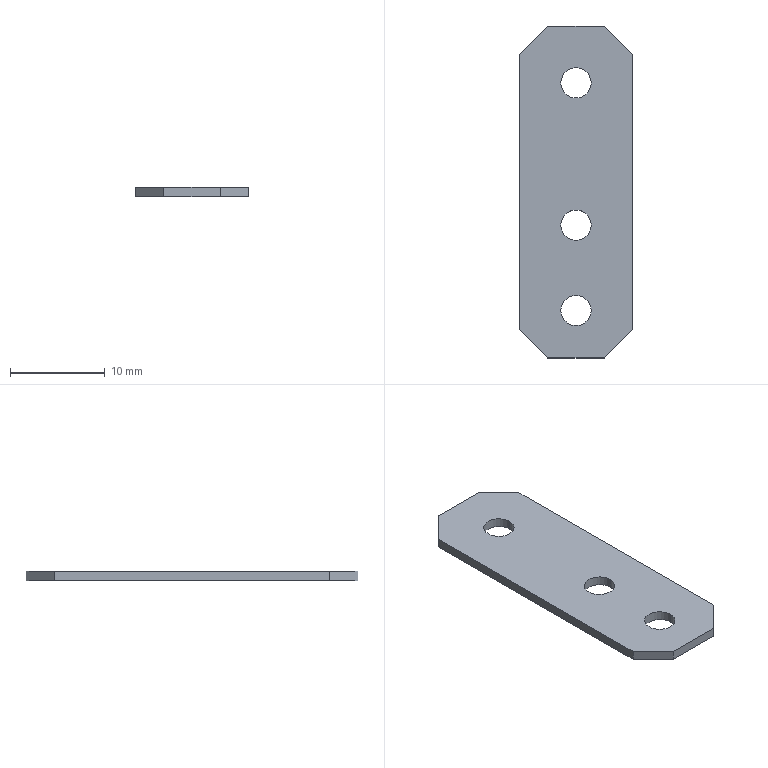Part | SolidWorks | features BaseBody 1 | 1 solid | 16 faces | box 12 x 35 x 1 mm | volume 377.873 mm3 | plane 10 | cylinder 6 | commonest cylinder face diameters 3.2 x6
STEP:
#1=CARTESIAN_POINT('',(1.6,-12.5,-1.));
#2=VERTEX_POINT('',#1);
#3=CARTESIAN_POINT('',(-1.6,-12.5,-1.));
#4=VERTEX_POINT('',#3);
#5=CARTESIAN_POINT('',(0.,-12.5,-1.));
#6=DIRECTION('',(0.,0.,-1.));
#7=DIRECTION('',(1.,0.,0.));
#8=AXIS2_PLACEMENT_3D('',#5,#6,#7);
#9=CIRCLE('',#8,1.6);
#10=EDGE_CURVE('',#2,#4,#9,.T.);
#11=ORIENTED_EDGE('',*,*,#10,.T.);
#12=CARTESIAN_POINT('',(-1.6,-12.5,0.));
#13=VERTEX_POINT('',#12);
#14=CARTESIAN_POINT('',(-1.6,-12.5,-1.));
#15=DIRECTION('',(0.,0.,1.));
#16=VECTOR('',#15,1000.);
#17=LINE('',#14,#16);
#18=EDGE_CURVE('',#4,#13,#17,.T.);
#19=ORIENTED_EDGE('',*,*,#18,.T.);
#20=CARTESIAN_POINT('',(1.6,-12.5,0.));
#21=VERTEX_POINT('',#20);
#22=CARTESIAN_POINT('',(0.,-12.5,0.));
#23=DIRECTION('',(0.,0.,1.));
#24=DIRECTION('',(1.,0.,0.));
#25=AXIS2_PLACEMENT_3D('',#22,#23,#24);
#26=CIRCLE('',#25,1.6);
#27=EDGE_CURVE('',#13,#21,#26,.T.);
#28=ORIENTED_EDGE('',*,*,#27,.T.);
#29=CARTESIAN_POINT('',(1.6,-12.5,-1.));
#30=DIRECTION('',(0.,0.,1.));
#31=VECTOR('',#30,1000.);
#32=LINE('',#29,#31);
#33=EDGE_CURVE('',#2,#21,#32,.T.);
#34=ORIENTED_EDGE('',*,*,#33,.F.);
#35=EDGE_LOOP('',(#11,#19,#28,#34));
#36=FACE_OUTER_BOUND('',#35,.T.);
#37=CARTESIAN_POINT('',(0.,-12.5,-1.));
#38=DIRECTION('',(0.,0.,1.));
#39=DIRECTION('',(1.,0.,0.));
#40=AXIS2_PLACEMENT_3D('',#37,#38,#39);
#41=CYLINDRICAL_SURFACE('',#40,1.6);
#42=ADVANCED_FACE('',(#36),#41,.F.);
#43=CARTESIAN_POINT('',(1.6,11.5,-1.));
#44=VERTEX_POINT('',#43);
#45=CARTESIAN_POINT('',(-1.6,11.5,-1.));
#46=VERTEX_POINT('',#45);
#47=CARTESIAN_POINT('',(0.,11.5,-1.));
#48=DIRECTION('',(0.,0.,-1.));
#49=DIRECTION('',(1.,0.,0.));
#50=AXIS2_PLACEMENT_3D('',#47,#48,#49);
#51=CIRCLE('',#50,1.6);
#52=EDGE_CURVE('',#44,#46,#51,.T.);
#53=ORIENTED_EDGE('',*,*,#52,.T.);
#54=CARTESIAN_POINT('',(-1.6,11.5,0.));
#55=VERTEX_POINT('',#54);
#56=CARTESIAN_POINT('',(-1.6,11.5,-1.));
#57=DIRECTION('',(0.,0.,1.));
#58=VECTOR('',#57,1000.);
#59=LINE('',#56,#58);
#60=EDGE_CURVE('',#46,#55,#59,.T.);
#61=ORIENTED_EDGE('',*,*,#60,.T.);
#62=CARTESIAN_POINT('',(1.6,11.5,0.));
#63=VERTEX_POINT('',#62);
#64=CARTESIAN_POINT('',(0.,11.5,0.));
#65=DIRECTION('',(0.,0.,-1.));
#66=DIRECTION('',(1.,0.,0.));
#67=AXIS2_PLACEMENT_3D('',#64,#65,#66);
#68=CIRCLE('',#67,1.6);
#69=EDGE_CURVE('',#63,#55,#68,.T.);
#70=ORIENTED_EDGE('',*,*,#69,.F.);
#71=CARTESIAN_POINT('',(1.6,11.5,-1.));
#72=DIRECTION('',(0.,0.,1.));
#73=VECTOR('',#72,1000.);
#74=LINE('',#71,#73);
#75=EDGE_CURVE('',#44,#63,#74,.T.);
#76=ORIENTED_EDGE('',*,*,#75,.F.);
#77=EDGE_LOOP('',(#53,#61,#70,#76));
#78=FACE_OUTER_BOUND('',#77,.T.);
#79=CARTESIAN_POINT('',(0.,11.5,-1.));
#80=DIRECTION('',(0.,0.,1.));
#81=DIRECTION('',(1.,0.,0.));
#82=AXIS2_PLACEMENT_3D('',#79,#80,#81);
#83=CYLINDRICAL_SURFACE('',#82,1.6);
#84=ADVANCED_FACE('',(#78),#83,.F.);
#85=CARTESIAN_POINT('',(1.6,-3.5,-1.));
#86=VERTEX_POINT('',#85);
#87=CARTESIAN_POINT('',(-1.6,-3.5,-1.));
#88=VERTEX_POINT('',#87);
#89=CARTESIAN_POINT('',(0.,-3.5,-1.));
#90=DIRECTION('',(0.,0.,-1.));
#91=DIRECTION('',(1.,0.,0.));
#92=AXIS2_PLACEMENT_3D('',#89,#90,#91);
#93=CIRCLE('',#92,1.6);
#94=EDGE_CURVE('',#86,#88,#93,.T.);
#95=ORIENTED_EDGE('',*,*,#94,.T.);
#96=CARTESIAN_POINT('',(-1.6,-3.5,0.));
#97=VERTEX_POINT('',#96);
#98=CARTESIAN_POINT('',(-1.6,-3.5,-1.));
#99=DIRECTION('',(0.,0.,1.));
#100=VECTOR('',#99,1000.);
#101=LINE('',#98,#100);
#102=EDGE_CURVE('',#88,#97,#101,.T.);
#103=ORIENTED_EDGE('',*,*,#102,.T.);
#104=CARTESIAN_POINT('',(1.6,-3.5,0.));
#105=VERTEX_POINT('',#104);
#106=CARTESIAN_POINT('',(0.,-3.5,0.));
#107=DIRECTION('',(0.,0.,-1.));
#108=DIRECTION('',(1.,0.,0.));
#109=AXIS2_PLACEMENT_3D('',#106,#107,#108);
#110=CIRCLE('',#109,1.6);
#111=EDGE_CURVE('',#105,#97,#110,.T.);
#112=ORIENTED_EDGE('',*,*,#111,.F.);
#113=CARTESIAN_POINT('',(1.6,-3.5,-1.));
#114=DIRECTION('',(0.,0.,1.));
#115=VECTOR('',#114,1000.);
#116=LINE('',#113,#115);
#117=EDGE_CURVE('',#86,#105,#116,.T.);
#118=ORIENTED_EDGE('',*,*,#117,.F.);
#119=EDGE_LOOP('',(#95,#103,#112,#118));
#120=FACE_OUTER_BOUND('',#119,.T.);
#121=CARTESIAN_POINT('',(0.,-3.5,-1.));
#122=DIRECTION('',(0.,0.,1.));
#123=DIRECTION('',(1.,0.,0.));
#124=AXIS2_PLACEMENT_3D('',#121,#122,#123);
#125=CYLINDRICAL_SURFACE('',#124,1.6);
#126=ADVANCED_FACE('',(#120),#125,.F.);
#127=ORIENTED_EDGE('',*,*,#18,.F.);
#128=CARTESIAN_POINT('',(0.,-12.5,-1.));
#129=DIRECTION('',(0.,0.,-1.));
#130=DIRECTION('',(1.,0.,0.));
#131=AXIS2_PLACEMENT_3D('',#128,#129,#130);
#132=CIRCLE('',#131,1.6);
#133=EDGE_CURVE('',#4,#2,#132,.T.);
#134=ORIENTED_EDGE('',*,*,#133,.T.);
#135=ORIENTED_EDGE('',*,*,#33,.T.);
#136=CARTESIAN_POINT('',(0.,-12.5,0.));
#137=DIRECTION('',(0.,0.,1.));
#138=DIRECTION('',(1.,0.,0.));
#139=AXIS2_PLACEMENT_3D('',#136,#137,#138);
#140=CIRCLE('',#139,1.6);
#141=EDGE_CURVE('',#21,#13,#140,.T.);
#142=ORIENTED_EDGE('',*,*,#141,.T.);
#143=EDGE_LOOP('',(#127,#134,#135,#142));
#144=FACE_OUTER_BOUND('',#143,.T.);
#145=CARTESIAN_POINT('',(0.,-12.5,-1.));
#146=DIRECTION('',(0.,0.,1.));
#147=DIRECTION('',(1.,0.,0.));
#148=AXIS2_PLACEMENT_3D('',#145,#146,#147);
#149=CYLINDRICAL_SURFACE('',#148,1.6);
#150=ADVANCED_FACE('',(#144),#149,.F.);
#151=ORIENTED_EDGE('',*,*,#69,.T.);
#152=CARTESIAN_POINT('',(0.,11.5,0.));
#153=DIRECTION('',(0.,0.,-1.));
#154=DIRECTION('',(1.,0.,0.));
#155=AXIS2_PLACEMENT_3D('',#152,#153,#154);
#156=CIRCLE('',#155,1.6);
#157=EDGE_CURVE('',#55,#63,#156,.T.);
#158=ORIENTED_EDGE('',*,*,#157,.T.);
#159=EDGE_LOOP('',(#151,#158));
#160=FACE_BOUND('',#159,.T.);
#161=ORIENTED_EDGE('',*,*,#111,.T.);
#162=CARTESIAN_POINT('',(0.,-3.5,0.));
#163=DIRECTION('',(0.,0.,-1.));
#164=DIRECTION('',(1.,0.,0.));
#165=AXIS2_PLACEMENT_3D('',#162,#163,#164);
#166=CIRCLE('',#165,1.6);
#167=EDGE_CURVE('',#97,#105,#166,.T.);
#168=ORIENTED_EDGE('',*,*,#167,.T.);
#169=EDGE_LOOP('',(#161,#168));
#170=FACE_BOUND('',#169,.T.);
#171=ORIENTED_EDGE('',*,*,#141,.F.);
#172=ORIENTED_EDGE('',*,*,#27,.F.);
#173=EDGE_LOOP('',(#171,#172));
#174=FACE_BOUND('',#173,.T.);
#175=CARTESIAN_POINT('',(6.,-14.5,0.));
#176=VERTEX_POINT('',#175);
#177=CARTESIAN_POINT('',(6.,14.5,0.));
#178=VERTEX_POINT('',#177);
#179=CARTESIAN_POINT('',(6.,0.,0.));
#180=DIRECTION('',(0.,1.,0.));
#181=VECTOR('',#180,1000.);
#182=LINE('',#179,#181);
#183=EDGE_CURVE('',#176,#178,#182,.T.);
#184=ORIENTED_EDGE('',*,*,#183,.T.);
#185=CARTESIAN_POINT('',(3.,17.5,0.));
#186=VERTEX_POINT('',#185);
#187=CARTESIAN_POINT('',(6.,14.5,0.));
#188=DIRECTION('',(-0.7071,0.7071,0.));
#189=VECTOR('',#188,1000.);
#190=LINE('',#187,#189);
#191=EDGE_CURVE('',#178,#186,#190,.T.);
#192=ORIENTED_EDGE('',*,*,#191,.T.);
#193=CARTESIAN_POINT('',(-3.,17.5,0.));
#194=VERTEX_POINT('',#193);
#195=CARTESIAN_POINT('',(0.,17.5,0.));
#196=DIRECTION('',(-1.,0.,0.));
#197=VECTOR('',#196,1000.);
#198=LINE('',#195,#197);
#199=EDGE_CURVE('',#186,#194,#198,.T.);
#200=ORIENTED_EDGE('',*,*,#199,.T.);
#201=CARTESIAN_POINT('',(-6.,14.5,0.));
#202=VERTEX_POINT('',#201);
#203=CARTESIAN_POINT('',(-3.,17.5,0.));
#204=DIRECTION('',(-0.7071,-0.7071,0.));
#205=VECTOR('',#204,1000.);
#206=LINE('',#203,#205);
#207=EDGE_CURVE('',#194,#202,#206,.T.);
#208=ORIENTED_EDGE('',*,*,#207,.T.);
#209=CARTESIAN_POINT('',(-6.,-14.5,0.));
#210=VERTEX_POINT('',#209);
#211=CARTESIAN_POINT('',(-6.,0.,0.));
#212=DIRECTION('',(0.,-1.,0.));
#213=VECTOR('',#212,1000.);
#214=LINE('',#211,#213);
#215=EDGE_CURVE('',#202,#210,#214,.T.);
#216=ORIENTED_EDGE('',*,*,#215,.T.);
#217=CARTESIAN_POINT('',(-3.,-17.5,0.));
#218=VERTEX_POINT('',#217);
#219=CARTESIAN_POINT('',(-6.,-14.5,0.));
#220=DIRECTION('',(0.7071,-0.7071,0.));
#221=VECTOR('',#220,1000.);
#222=LINE('',#219,#221);
#223=EDGE_CURVE('',#210,#218,#222,.T.);
#224=ORIENTED_EDGE('',*,*,#223,.T.);
#225=CARTESIAN_POINT('',(3.,-17.5,0.));
#226=VERTEX_POINT('',#225);
#227=CARTESIAN_POINT('',(0.,-17.5,0.));
#228=DIRECTION('',(1.,0.,0.));
#229=VECTOR('',#228,1000.);
#230=LINE('',#227,#229);
#231=EDGE_CURVE('',#218,#226,#230,.T.);
#232=ORIENTED_EDGE('',*,*,#231,.T.);
#233=CARTESIAN_POINT('',(3.,-17.5,0.));
#234=DIRECTION('',(0.7071,0.7071,0.));
#235=VECTOR('',#234,1000.);
#236=LINE('',#233,#235);
#237=EDGE_CURVE('',#226,#176,#236,.T.);
#238=ORIENTED_EDGE('',*,*,#237,.T.);
#239=EDGE_LOOP('',(#184,#192,#200,#208,#216,#224,#232,#238));
#240=FACE_OUTER_BOUND('',#239,.T.);
#241=CARTESIAN_POINT('',(-6.,-17.5,0.));
#242=DIRECTION('',(0.,0.,1.));
#243=DIRECTION('',(1.,0.,0.));
#244=AXIS2_PLACEMENT_3D('',#241,#242,#243);
#245=PLANE('',#244);
#246=ADVANCED_FACE('',(#160,#170,#174,#240),#245,.T.);
#247=ORIENTED_EDGE('',*,*,#52,.F.);
#248=CARTESIAN_POINT('',(0.,11.5,-1.));
#249=DIRECTION('',(0.,0.,-1.));
#250=DIRECTION('',(1.,0.,0.));
#251=AXIS2_PLACEMENT_3D('',#248,#249,#250);
#252=CIRCLE('',#251,1.6);
#253=EDGE_CURVE('',#46,#44,#252,.T.);
#254=ORIENTED_EDGE('',*,*,#253,.F.);
#255=EDGE_LOOP('',(#247,#254));
#256=FACE_BOUND('',#255,.T.);
#257=ORIENTED_EDGE('',*,*,#94,.F.);
#258=CARTESIAN_POINT('',(0.,-3.5,-1.));
#259=DIRECTION('',(0.,0.,-1.));
#260=DIRECTION('',(1.,0.,0.));
#261=AXIS2_PLACEMENT_3D('',#258,#259,#260);
#262=CIRCLE('',#261,1.6);
#263=EDGE_CURVE('',#88,#86,#262,.T.);
#264=ORIENTED_EDGE('',*,*,#263,.F.);
#265=EDGE_LOOP('',(#257,#264));
#266=FACE_BOUND('',#265,.T.);
#267=ORIENTED_EDGE('',*,*,#10,.F.);
#268=ORIENTED_EDGE('',*,*,#133,.F.);
#269=EDGE_LOOP('',(#267,#268));
#270=FACE_BOUND('',#269,.T.);
#271=CARTESIAN_POINT('',(6.,14.5,-1.));
#272=VERTEX_POINT('',#271);
#273=CARTESIAN_POINT('',(3.,17.5,-1.));
#274=VERTEX_POINT('',#273);
#275=CARTESIAN_POINT('',(6.,14.5,-1.));
#276=DIRECTION('',(-0.7071,0.7071,0.));
#277=VECTOR('',#276,1000.);
#278=LINE('',#275,#277);
#279=EDGE_CURVE('',#272,#274,#278,.T.);
#280=ORIENTED_EDGE('',*,*,#279,.F.);
#281=CARTESIAN_POINT('',(6.,-14.5,-1.));
#282=VERTEX_POINT('',#281);
#283=CARTESIAN_POINT('',(6.,0.,-1.));
#284=DIRECTION('',(0.,1.,0.));
#285=VECTOR('',#284,1000.);
#286=LINE('',#283,#285);
#287=EDGE_CURVE('',#282,#272,#286,.T.);
#288=ORIENTED_EDGE('',*,*,#287,.F.);
#289=CARTESIAN_POINT('',(3.,-17.5,-1.));
#290=VERTEX_POINT('',#289);
#291=CARTESIAN_POINT('',(3.,-17.5,-1.));
#292=DIRECTION('',(0.7071,0.7071,0.));
#293=VECTOR('',#292,1000.);
#294=LINE('',#291,#293);
#295=EDGE_CURVE('',#290,#282,#294,.T.);
#296=ORIENTED_EDGE('',*,*,#295,.F.);
#297=CARTESIAN_POINT('',(-3.,-17.5,-1.));
#298=VERTEX_POINT('',#297);
#299=CARTESIAN_POINT('',(0.,-17.5,-1.));
#300=DIRECTION('',(1.,0.,0.));
#301=VECTOR('',#300,1000.);
#302=LINE('',#299,#301);
#303=EDGE_CURVE('',#298,#290,#302,.T.);
#304=ORIENTED_EDGE('',*,*,#303,.F.);
#305=CARTESIAN_POINT('',(-6.,-14.5,-1.));
#306=VERTEX_POINT('',#305);
#307=CARTESIAN_POINT('',(-6.,-14.5,-1.));
#308=DIRECTION('',(0.7071,-0.7071,0.));
#309=VECTOR('',#308,1000.);
#310=LINE('',#307,#309);
#311=EDGE_CURVE('',#306,#298,#310,.T.);
#312=ORIENTED_EDGE('',*,*,#311,.F.);
#313=CARTESIAN_POINT('',(-6.,14.5,-1.));
#314=VERTEX_POINT('',#313);
#315=CARTESIAN_POINT('',(-6.,0.,-1.));
#316=DIRECTION('',(0.,-1.,0.));
#317=VECTOR('',#316,1000.);
#318=LINE('',#315,#317);
#319=EDGE_CURVE('',#314,#306,#318,.T.);
#320=ORIENTED_EDGE('',*,*,#319,.F.);
#321=CARTESIAN_POINT('',(-3.,17.5,-1.));
#322=VERTEX_POINT('',#321);
#323=CARTESIAN_POINT('',(-3.,17.5,-1.));
#324=DIRECTION('',(-0.7071,-0.7071,0.));
#325=VECTOR('',#324,1000.);
#326=LINE('',#323,#325);
#327=EDGE_CURVE('',#322,#314,#326,.T.);
#328=ORIENTED_EDGE('',*,*,#327,.F.);
#329=CARTESIAN_POINT('',(0.,17.5,-1.));
#330=DIRECTION('',(-1.,0.,0.));
#331=VECTOR('',#330,1000.);
#332=LINE('',#329,#331);
#333=EDGE_CURVE('',#274,#322,#332,.T.);
#334=ORIENTED_EDGE('',*,*,#333,.F.);
#335=EDGE_LOOP('',(#280,#288,#296,#304,#312,#320,#328,#334));
#336=FACE_OUTER_BOUND('',#335,.T.);
#337=CARTESIAN_POINT('',(-6.,-17.5,-1.));
#338=DIRECTION('',(0.,0.,1.));
#339=DIRECTION('',(1.,0.,0.));
#340=AXIS2_PLACEMENT_3D('',#337,#338,#339);
#341=PLANE('',#340);
#342=ADVANCED_FACE('',(#256,#266,#270,#336),#341,.F.);
#343=ORIENTED_EDGE('',*,*,#60,.F.);
#344=ORIENTED_EDGE('',*,*,#253,.T.);
#345=ORIENTED_EDGE('',*,*,#75,.T.);
#346=ORIENTED_EDGE('',*,*,#157,.F.);
#347=EDGE_LOOP('',(#343,#344,#345,#346));
#348=FACE_OUTER_BOUND('',#347,.T.);
#349=CARTESIAN_POINT('',(0.,11.5,-1.));
#350=DIRECTION('',(0.,0.,1.));
#351=DIRECTION('',(1.,0.,0.));
#352=AXIS2_PLACEMENT_3D('',#349,#350,#351);
#353=CYLINDRICAL_SURFACE('',#352,1.6);
#354=ADVANCED_FACE('',(#348),#353,.F.);
#355=ORIENTED_EDGE('',*,*,#102,.F.);
#356=ORIENTED_EDGE('',*,*,#263,.T.);
#357=ORIENTED_EDGE('',*,*,#117,.T.);
#358=ORIENTED_EDGE('',*,*,#167,.F.);
#359=EDGE_LOOP('',(#355,#356,#357,#358));
#360=FACE_OUTER_BOUND('',#359,.T.);
#361=CARTESIAN_POINT('',(0.,-3.5,-1.));
#362=DIRECTION('',(0.,0.,1.));
#363=DIRECTION('',(1.,0.,0.));
#364=AXIS2_PLACEMENT_3D('',#361,#362,#363);
#365=CYLINDRICAL_SURFACE('',#364,1.6);
#366=ADVANCED_FACE('',(#360),#365,.F.);
#367=ORIENTED_EDGE('',*,*,#279,.T.);
#368=CARTESIAN_POINT('',(3.,17.5,-0.5));
#369=DIRECTION('',(0.,0.,1.));
#370=VECTOR('',#369,1000.);
#371=LINE('',#368,#370);
#372=EDGE_CURVE('',#274,#186,#371,.T.);
#373=ORIENTED_EDGE('',*,*,#372,.T.);
#374=ORIENTED_EDGE('',*,*,#191,.F.);
#375=CARTESIAN_POINT('',(6.,14.5,-0.5));
#376=DIRECTION('',(0.,0.,-1.));
#377=VECTOR('',#376,1000.);
#378=LINE('',#375,#377);
#379=EDGE_CURVE('',#178,#272,#378,.T.);
#380=ORIENTED_EDGE('',*,*,#379,.T.);
#381=EDGE_LOOP('',(#367,#373,#374,#380));
#382=FACE_OUTER_BOUND('',#381,.T.);
#383=CARTESIAN_POINT('',(6.,14.5,-1.));
#384=DIRECTION('',(0.7071,0.7071,0.));
#385=DIRECTION('',(-0.7071,0.7071,0.));
#386=AXIS2_PLACEMENT_3D('',#383,#384,#385);
#387=PLANE('',#386);
#388=ADVANCED_FACE('',(#382),#387,.T.);
#389=ORIENTED_EDGE('',*,*,#287,.T.);
#390=ORIENTED_EDGE('',*,*,#379,.F.);
#391=ORIENTED_EDGE('',*,*,#183,.F.);
#392=CARTESIAN_POINT('',(6.,-14.5,-0.5));
#393=DIRECTION('',(0.,0.,-1.));
#394=VECTOR('',#393,1000.);
#395=LINE('',#392,#394);
#396=EDGE_CURVE('',#176,#282,#395,.T.);
#397=ORIENTED_EDGE('',*,*,#396,.T.);
#398=EDGE_LOOP('',(#389,#390,#391,#397));
#399=FACE_OUTER_BOUND('',#398,.T.);
#400=CARTESIAN_POINT('',(6.,-14.5,0.));
#401=DIRECTION('',(1.,0.,0.));
#402=DIRECTION('',(0.,0.,-1.));
#403=AXIS2_PLACEMENT_3D('',#400,#401,#402);
#404=PLANE('',#403);
#405=ADVANCED_FACE('',(#399),#404,.T.);
#406=ORIENTED_EDGE('',*,*,#295,.T.);
#407=ORIENTED_EDGE('',*,*,#396,.F.);
#408=ORIENTED_EDGE('',*,*,#237,.F.);
#409=CARTESIAN_POINT('',(3.,-17.5,-0.5));
#410=DIRECTION('',(0.,0.,-1.));
#411=VECTOR('',#410,1000.);
#412=LINE('',#409,#411);
#413=EDGE_CURVE('',#226,#290,#412,.T.);
#414=ORIENTED_EDGE('',*,*,#413,.T.);
#415=EDGE_LOOP('',(#406,#407,#408,#414));
#416=FACE_OUTER_BOUND('',#415,.T.);
#417=CARTESIAN_POINT('',(3.,-17.5,-1.));
#418=DIRECTION('',(0.7071,-0.7071,0.));
#419=DIRECTION('',(0.7071,0.7071,0.));
#420=AXIS2_PLACEMENT_3D('',#417,#418,#419);
#421=PLANE('',#420);
#422=ADVANCED_FACE('',(#416),#421,.T.);
#423=ORIENTED_EDGE('',*,*,#303,.T.);
#424=ORIENTED_EDGE('',*,*,#413,.F.);
#425=ORIENTED_EDGE('',*,*,#231,.F.);
#426=CARTESIAN_POINT('',(-3.,-17.5,-0.5));
#427=DIRECTION('',(0.,0.,-1.));
#428=VECTOR('',#427,1000.);
#429=LINE('',#426,#428);
#430=EDGE_CURVE('',#218,#298,#429,.T.);
#431=ORIENTED_EDGE('',*,*,#430,.T.);
#432=EDGE_LOOP('',(#423,#424,#425,#431));
#433=FACE_OUTER_BOUND('',#432,.T.);
#434=CARTESIAN_POINT('',(-3.,-17.5,-1.));
#435=DIRECTION('',(0.,-1.,0.));
#436=DIRECTION('',(1.,0.,0.));
#437=AXIS2_PLACEMENT_3D('',#434,#435,#436);
#438=PLANE('',#437);
#439=ADVANCED_FACE('',(#433),#438,.T.);
#440=ORIENTED_EDGE('',*,*,#311,.T.);
#441=ORIENTED_EDGE('',*,*,#430,.F.);
#442=ORIENTED_EDGE('',*,*,#223,.F.);
#443=CARTESIAN_POINT('',(-6.,-14.5,-0.5));
#444=DIRECTION('',(0.,0.,-1.));
#445=VECTOR('',#444,1000.);
#446=LINE('',#443,#445);
#447=EDGE_CURVE('',#210,#306,#446,.T.);
#448=ORIENTED_EDGE('',*,*,#447,.T.);
#449=EDGE_LOOP('',(#440,#441,#442,#448));
#450=FACE_OUTER_BOUND('',#449,.T.);
#451=CARTESIAN_POINT('',(-6.,-14.5,-1.));
#452=DIRECTION('',(-0.7071,-0.7071,0.));
#453=DIRECTION('',(0.7071,-0.7071,0.));
#454=AXIS2_PLACEMENT_3D('',#451,#452,#453);
#455=PLANE('',#454);
#456=ADVANCED_FACE('',(#450),#455,.T.);
#457=ORIENTED_EDGE('',*,*,#319,.T.);
#458=ORIENTED_EDGE('',*,*,#447,.F.);
#459=ORIENTED_EDGE('',*,*,#215,.F.);
#460=CARTESIAN_POINT('',(-6.,14.5,-0.5));
#461=DIRECTION('',(0.,0.,-1.));
#462=VECTOR('',#461,1000.);
#463=LINE('',#460,#462);
#464=EDGE_CURVE('',#202,#314,#463,.T.);
#465=ORIENTED_EDGE('',*,*,#464,.T.);
#466=EDGE_LOOP('',(#457,#458,#459,#465));
#467=FACE_OUTER_BOUND('',#466,.T.);
#468=CARTESIAN_POINT('',(-6.,14.5,-1.));
#469=DIRECTION('',(-1.,0.,0.));
#470=DIRECTION('',(0.,-1.,0.));
#471=AXIS2_PLACEMENT_3D('',#468,#469,#470);
#472=PLANE('',#471);
#473=ADVANCED_FACE('',(#467),#472,.T.);
#474=ORIENTED_EDGE('',*,*,#327,.T.);
#475=ORIENTED_EDGE('',*,*,#464,.F.);
#476=ORIENTED_EDGE('',*,*,#207,.F.);
#477=CARTESIAN_POINT('',(-3.,17.5,-0.5));
#478=DIRECTION('',(0.,0.,-1.));
#479=VECTOR('',#478,1000.);
#480=LINE('',#477,#479);
#481=EDGE_CURVE('',#194,#322,#480,.T.);
#482=ORIENTED_EDGE('',*,*,#481,.T.);
#483=EDGE_LOOP('',(#474,#475,#476,#482));
#484=FACE_OUTER_BOUND('',#483,.T.);
#485=CARTESIAN_POINT('',(-3.,17.5,-1.));
#486=DIRECTION('',(-0.7071,0.7071,0.));
#487=DIRECTION('',(-0.7071,-0.7071,0.));
#488=AXIS2_PLACEMENT_3D('',#485,#486,#487);
#489=PLANE('',#488);
#490=ADVANCED_FACE('',(#484),#489,.T.);
#491=ORIENTED_EDGE('',*,*,#333,.T.);
#492=ORIENTED_EDGE('',*,*,#481,.F.);
#493=ORIENTED_EDGE('',*,*,#199,.F.);
#494=ORIENTED_EDGE('',*,*,#372,.F.);
#495=EDGE_LOOP('',(#491,#492,#493,#494));
#496=FACE_OUTER_BOUND('',#495,.T.);
#497=CARTESIAN_POINT('',(3.,17.5,-1.));
#498=DIRECTION('',(0.,1.,0.));
#499=DIRECTION('',(-1.,0.,0.));
#500=AXIS2_PLACEMENT_3D('',#497,#498,#499);
#501=PLANE('',#500);
#502=ADVANCED_FACE('',(#496),#501,.T.);
#503=CLOSED_SHELL('',(#42,#84,#126,#150,#246,#342,#354,#366,#388,#405,#422,#439,#456,#473,#490,#502));
#504=MANIFOLD_SOLID_BREP('',#503);
#505=CARTESIAN_POINT('',(0.,0.,0.));
#506=DIRECTION('',(0.,0.,1.));
#507=DIRECTION('',(1.,0.,0.));
#508=AXIS2_PLACEMENT_3D('',#505,#506,#507);
#509=(LENGTH_UNIT()NAMED_UNIT(*)SI_UNIT(.MILLI.,.METRE.));
#510=UNCERTAINTY_MEASURE_WITH_UNIT(LENGTH_MEASURE(0.00001),#509,'','');
#511=(NAMED_UNIT(*)PLANE_ANGLE_UNIT()SI_UNIT($,.RADIAN.));
#512=(NAMED_UNIT(*)SI_UNIT($,.STERADIAN.)SOLID_ANGLE_UNIT());
#513=(GEOMETRIC_REPRESENTATION_CONTEXT(3)GLOBAL_UNCERTAINTY_ASSIGNED_CONTEXT((#510))GLOBAL_UNIT_ASSIGNED_CONTEXT((#509,#511,#512))REPRESENTATION_CONTEXT('',''));
#514=ADVANCED_BREP_SHAPE_REPRESENTATION('',(#504,#508),#513);